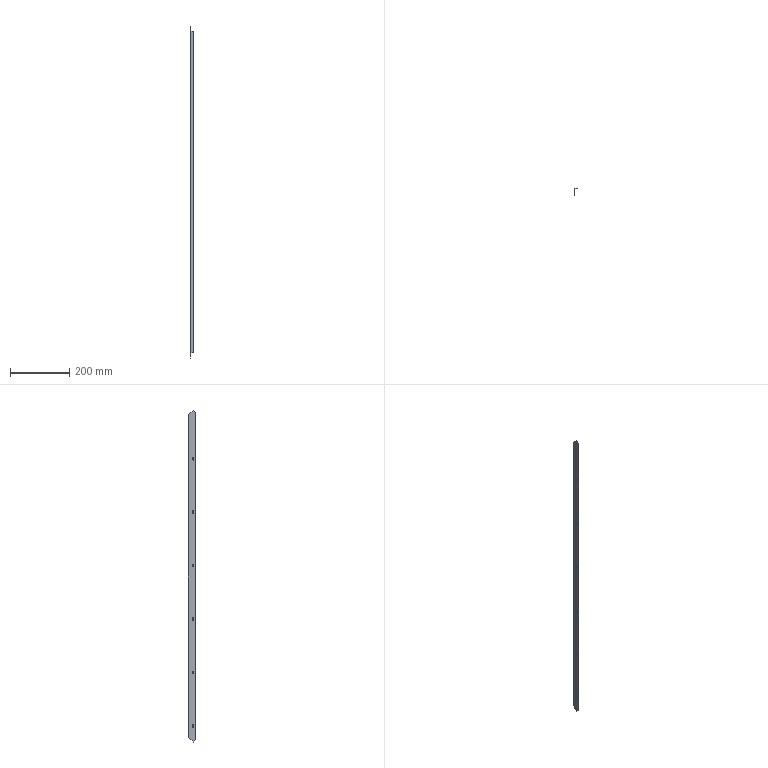Part | STEP file | RJWD-DY-0102_X2_5DE667DC95E8_28 | 1 solid | 52 faces | box 10 x 25 x 1118 mm | volume 36787 mm3 | plane 36 | cylinder 14 | spline 2 | commonest cylinder face diameters 5 x12 0.4 x1 2.4 x1